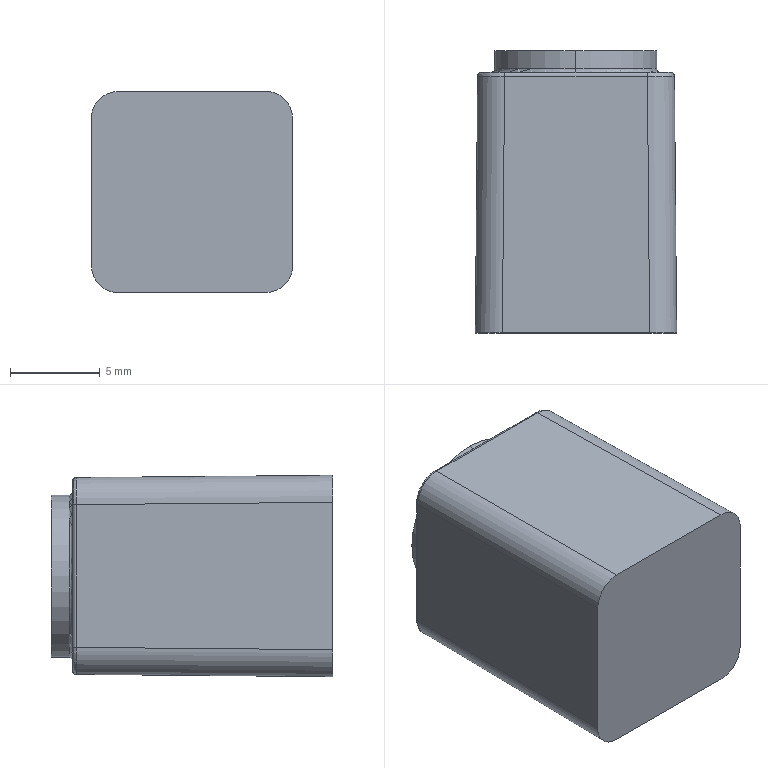Part | STEP file | 1 solid | 23 faces | box 11.23 x 15.729 x 11.23 mm | volume 1839 mm3 | cylinder 10 | plane 7 | spline 4 | torus 2 | commonest cylinder face diameters 0.402 x4 3.015 x4 9.045 x2